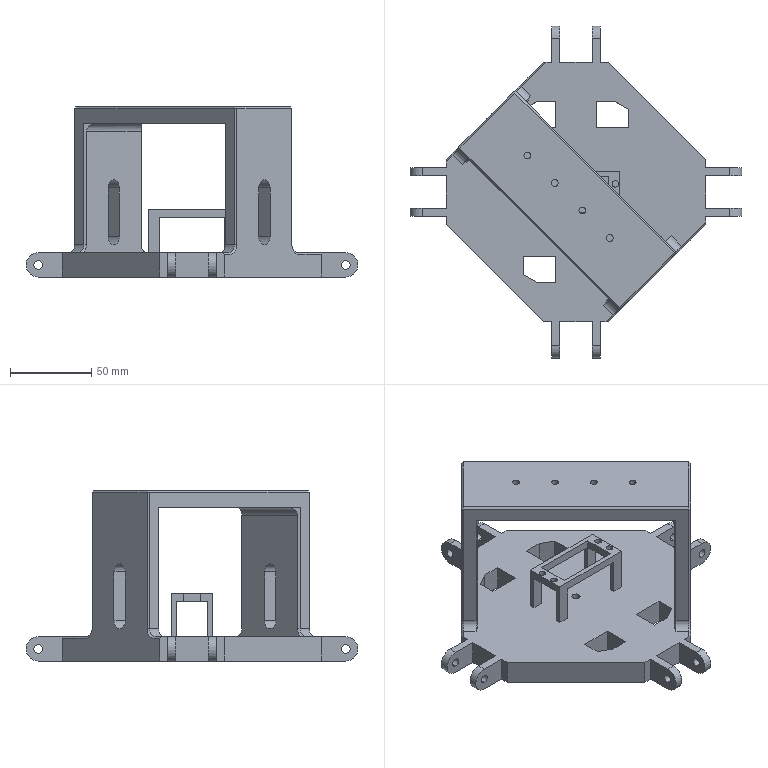Part | SolidWorks | features ICE 14, Fillet 2, MirrorPattern 2, MoveFace 2, Chamfer 1, Extrusion 1, HoleWzd 1 | 1 solid | 163 faces | box 205 x 205 x 105 mm | volume 416769 mm3 | plane 104 | cylinder 52 | cone 7 | commonest cylinder face diameters 5.2 x16 10 x10 4.1 x8 4.2 x8 15 x8 5 x2